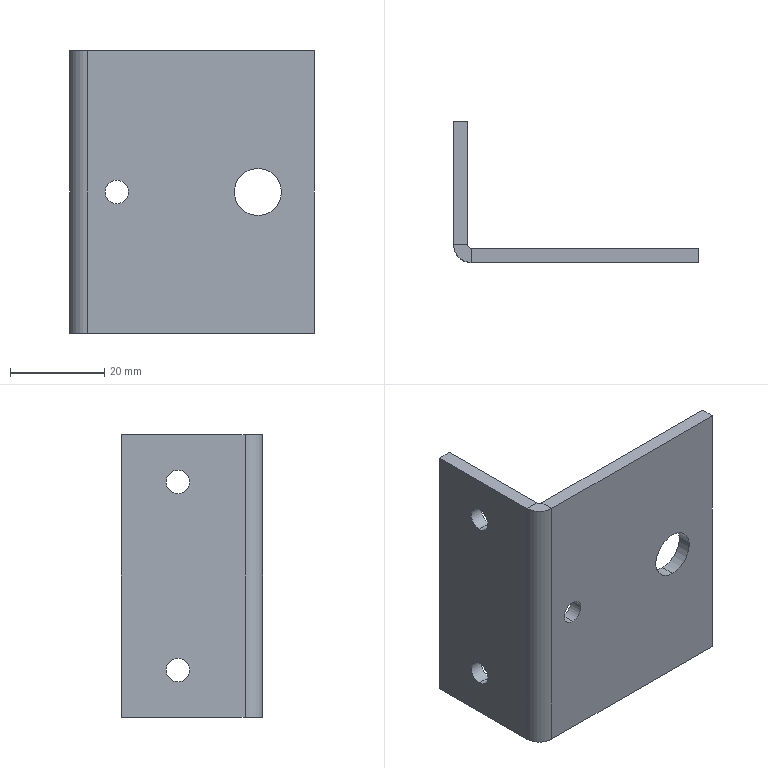Part | NX | features BREP 1 | 1 solid | 22 faces | box 52 x 30 x 60 mm | volume 13635 mm3 | plane 12 | cylinder 10 | commonest cylinder face diameters 5 x6 10 x2 1.473 x1 7.473 x1
STEP:
#1=CARTESIAN_POINT('',(-52.,18.,-22.5));
#2=VERTEX_POINT('',#1);
#3=CARTESIAN_POINT('',(-49.,18.,-22.5));
#4=VERTEX_POINT('',#3);
#5=CARTESIAN_POINT('',(-52.,18.,-22.5));
#6=DIRECTION('',(-1.,0.,0.));
#7=VECTOR('',#6,1000.);
#8=LINE('',#5,#7);
#9=EDGE_CURVE('',#2,#4,#8,.F.);
#10=ORIENTED_EDGE('',*,*,#9,.T.);
#11=CARTESIAN_POINT('',(-49.,18.,-17.5));
#12=VERTEX_POINT('',#11);
#13=CARTESIAN_POINT('',(-49.,18.,-20.));
#14=DIRECTION('',(-1.,0.,0.));
#15=DIRECTION('',(0.,-1.,0.));
#16=AXIS2_PLACEMENT_3D('',#13,#14,#15);
#17=CIRCLE('',#16,2.5);
#18=EDGE_CURVE('',#12,#4,#17,.T.);
#19=ORIENTED_EDGE('',*,*,#18,.F.);
#20=CARTESIAN_POINT('',(-52.,18.,-17.5));
#21=VERTEX_POINT('',#20);
#22=CARTESIAN_POINT('',(-52.,18.,-17.5));
#23=DIRECTION('',(-1.,0.,0.));
#24=VECTOR('',#23,1000.);
#25=LINE('',#22,#24);
#26=EDGE_CURVE('',#21,#12,#25,.F.);
#27=ORIENTED_EDGE('',*,*,#26,.F.);
#28=CARTESIAN_POINT('',(-52.,18.,-20.));
#29=DIRECTION('',(-1.,0.,0.));
#30=DIRECTION('',(0.,0.,1.));
#31=AXIS2_PLACEMENT_3D('',#28,#29,#30);
#32=CIRCLE('',#31,2.5);
#33=EDGE_CURVE('',#21,#2,#32,.T.);
#34=ORIENTED_EDGE('',*,*,#33,.T.);
#35=EDGE_LOOP('',(#10,#19,#27,#34));
#36=FACE_BOUND('',#35,.T.);
#37=CARTESIAN_POINT('',(-52.,18.,-20.));
#38=DIRECTION('',(-1.,0.,0.));
#39=DIRECTION('',(0.,0.,1.));
#40=AXIS2_PLACEMENT_3D('',#37,#38,#39);
#41=CYLINDRICAL_SURFACE('',#40,2.5);
#42=ADVANCED_FACE('',(#36),#41,.F.);
#43=CARTESIAN_POINT('',(-52.,18.,17.5));
#44=VERTEX_POINT('',#43);
#45=CARTESIAN_POINT('',(-49.,18.,17.5));
#46=VERTEX_POINT('',#45);
#47=CARTESIAN_POINT('',(-52.,18.,17.5));
#48=DIRECTION('',(-1.,0.,0.));
#49=VECTOR('',#48,1000.);
#50=LINE('',#47,#49);
#51=EDGE_CURVE('',#44,#46,#50,.F.);
#52=ORIENTED_EDGE('',*,*,#51,.T.);
#53=CARTESIAN_POINT('',(-49.,18.,22.5));
#54=VERTEX_POINT('',#53);
#55=CARTESIAN_POINT('',(-49.,18.,20.));
#56=DIRECTION('',(-1.,0.,0.));
#57=DIRECTION('',(0.,-1.,0.));
#58=AXIS2_PLACEMENT_3D('',#55,#56,#57);
#59=CIRCLE('',#58,2.5);
#60=EDGE_CURVE('',#54,#46,#59,.T.);
#61=ORIENTED_EDGE('',*,*,#60,.F.);
#62=CARTESIAN_POINT('',(-52.,18.,22.5));
#63=VERTEX_POINT('',#62);
#64=CARTESIAN_POINT('',(-52.,18.,22.5));
#65=DIRECTION('',(-1.,0.,0.));
#66=VECTOR('',#65,1000.);
#67=LINE('',#64,#66);
#68=EDGE_CURVE('',#63,#54,#67,.F.);
#69=ORIENTED_EDGE('',*,*,#68,.F.);
#70=CARTESIAN_POINT('',(-52.,18.,20.));
#71=DIRECTION('',(-1.,0.,0.));
#72=DIRECTION('',(0.,0.,1.));
#73=AXIS2_PLACEMENT_3D('',#70,#71,#72);
#74=CIRCLE('',#73,2.5);
#75=EDGE_CURVE('',#63,#44,#74,.T.);
#76=ORIENTED_EDGE('',*,*,#75,.T.);
#77=EDGE_LOOP('',(#52,#61,#69,#76));
#78=FACE_BOUND('',#77,.T.);
#79=CARTESIAN_POINT('',(-52.,18.,20.));
#80=DIRECTION('',(-1.,0.,0.));
#81=DIRECTION('',(0.,0.,1.));
#82=AXIS2_PLACEMENT_3D('',#79,#80,#81);
#83=CYLINDRICAL_SURFACE('',#82,2.5);
#84=ADVANCED_FACE('',(#78),#83,.F.);
#85=CARTESIAN_POINT('',(-42.,3.,2.5));
#86=VERTEX_POINT('',#85);
#87=CARTESIAN_POINT('',(-42.,0.,2.5));
#88=VERTEX_POINT('',#87);
#89=CARTESIAN_POINT('',(-42.,0.,2.5));
#90=DIRECTION('',(0.,-1.,0.));
#91=VECTOR('',#90,1000.);
#92=LINE('',#89,#91);
#93=EDGE_CURVE('',#86,#88,#92,.T.);
#94=ORIENTED_EDGE('',*,*,#93,.F.);
#95=CARTESIAN_POINT('',(-42.,3.,-2.5));
#96=VERTEX_POINT('',#95);
#97=CARTESIAN_POINT('',(-42.,3.,0.));
#98=DIRECTION('',(0.,-1.,0.));
#99=DIRECTION('',(1.,0.,0.));
#100=AXIS2_PLACEMENT_3D('',#97,#98,#99);
#101=CIRCLE('',#100,2.5);
#102=EDGE_CURVE('',#96,#86,#101,.T.);
#103=ORIENTED_EDGE('',*,*,#102,.F.);
#104=CARTESIAN_POINT('',(-42.,0.,-2.5));
#105=VERTEX_POINT('',#104);
#106=CARTESIAN_POINT('',(-42.,0.,-2.5));
#107=DIRECTION('',(0.,-1.,0.));
#108=VECTOR('',#107,1000.);
#109=LINE('',#106,#108);
#110=EDGE_CURVE('',#96,#105,#109,.T.);
#111=ORIENTED_EDGE('',*,*,#110,.T.);
#112=CARTESIAN_POINT('',(-42.,0.,0.));
#113=DIRECTION('',(0.,-1.,0.));
#114=DIRECTION('',(0.,0.,-1.));
#115=AXIS2_PLACEMENT_3D('',#112,#113,#114);
#116=CIRCLE('',#115,2.5);
#117=EDGE_CURVE('',#105,#88,#116,.T.);
#118=ORIENTED_EDGE('',*,*,#117,.T.);
#119=EDGE_LOOP('',(#94,#103,#111,#118));
#120=FACE_BOUND('',#119,.T.);
#121=CARTESIAN_POINT('',(-42.,0.,0.));
#122=DIRECTION('',(0.,-1.,0.));
#123=DIRECTION('',(0.,0.,-1.));
#124=AXIS2_PLACEMENT_3D('',#121,#122,#123);
#125=CYLINDRICAL_SURFACE('',#124,2.5);
#126=ADVANCED_FACE('',(#120),#125,.F.);
#127=CARTESIAN_POINT('',(-12.,3.,-5.));
#128=VERTEX_POINT('',#127);
#129=CARTESIAN_POINT('',(-12.,0.,-5.));
#130=VERTEX_POINT('',#129);
#131=CARTESIAN_POINT('',(-12.,3.,-5.));
#132=DIRECTION('',(0.,1.,0.));
#133=VECTOR('',#132,1000.);
#134=LINE('',#131,#133);
#135=EDGE_CURVE('',#128,#130,#134,.F.);
#136=ORIENTED_EDGE('',*,*,#135,.T.);
#137=CARTESIAN_POINT('',(-12.,0.,5.));
#138=VERTEX_POINT('',#137);
#139=CARTESIAN_POINT('',(-12.,0.,0.));
#140=DIRECTION('',(0.,1.,0.));
#141=DIRECTION('',(0.,0.,1.));
#142=AXIS2_PLACEMENT_3D('',#139,#140,#141);
#143=CIRCLE('',#142,5.);
#144=EDGE_CURVE('',#138,#130,#143,.T.);
#145=ORIENTED_EDGE('',*,*,#144,.F.);
#146=CARTESIAN_POINT('',(-12.,3.,5.));
#147=VERTEX_POINT('',#146);
#148=CARTESIAN_POINT('',(-12.,3.,5.));
#149=DIRECTION('',(0.,1.,0.));
#150=VECTOR('',#149,1000.);
#151=LINE('',#148,#150);
#152=EDGE_CURVE('',#147,#138,#151,.F.);
#153=ORIENTED_EDGE('',*,*,#152,.F.);
#154=CARTESIAN_POINT('',(-12.,3.,0.));
#155=DIRECTION('',(0.,1.,0.));
#156=DIRECTION('',(0.,0.,1.));
#157=AXIS2_PLACEMENT_3D('',#154,#155,#156);
#158=CIRCLE('',#157,5.);
#159=EDGE_CURVE('',#147,#128,#158,.T.);
#160=ORIENTED_EDGE('',*,*,#159,.T.);
#161=EDGE_LOOP('',(#136,#145,#153,#160));
#162=FACE_BOUND('',#161,.T.);
#163=CARTESIAN_POINT('',(-12.,3.,0.));
#164=DIRECTION('',(0.,1.,0.));
#165=DIRECTION('',(0.,0.,1.));
#166=AXIS2_PLACEMENT_3D('',#163,#164,#165);
#167=CYLINDRICAL_SURFACE('',#166,5.);
#168=ADVANCED_FACE('',(#162),#167,.F.);
#169=CARTESIAN_POINT('',(-49.,3.737,-30.));
#170=VERTEX_POINT('',#169);
#171=CARTESIAN_POINT('',(-49.,30.,-30.));
#172=VERTEX_POINT('',#171);
#173=CARTESIAN_POINT('',(-49.,0.,-30.));
#174=DIRECTION('',(0.,1.,0.));
#175=VECTOR('',#174,1000.);
#176=LINE('',#173,#175);
#177=EDGE_CURVE('',#170,#172,#176,.T.);
#178=ORIENTED_EDGE('',*,*,#177,.F.);
#179=CARTESIAN_POINT('',(-52.,3.737,-30.));
#180=VERTEX_POINT('',#179);
#181=CARTESIAN_POINT('',(-49.,3.737,-30.));
#182=DIRECTION('',(-1.,0.,0.));
#183=VECTOR('',#182,1000.);
#184=LINE('',#181,#183);
#185=EDGE_CURVE('',#170,#180,#184,.T.);
#186=ORIENTED_EDGE('',*,*,#185,.T.);
#187=CARTESIAN_POINT('',(-52.,30.,-30.));
#188=VERTEX_POINT('',#187);
#189=CARTESIAN_POINT('',(-52.,0.,-30.));
#190=DIRECTION('',(0.,1.,0.));
#191=VECTOR('',#190,1000.);
#192=LINE('',#189,#191);
#193=EDGE_CURVE('',#180,#188,#192,.T.);
#194=ORIENTED_EDGE('',*,*,#193,.T.);
#195=CARTESIAN_POINT('',(-52.,30.,-30.));
#196=DIRECTION('',(1.,0.,0.));
#197=VECTOR('',#196,1000.);
#198=LINE('',#195,#197);
#199=EDGE_CURVE('',#188,#172,#198,.T.);
#200=ORIENTED_EDGE('',*,*,#199,.T.);
#201=EDGE_LOOP('',(#178,#186,#194,#200));
#202=FACE_BOUND('',#201,.T.);
#203=CARTESIAN_POINT('',(-48.263,3.737,-30.));
#204=DIRECTION('',(0.,0.,1.));
#205=DIRECTION('',(1.,0.,0.));
#206=AXIS2_PLACEMENT_3D('',#203,#204,#205);
#207=PLANE('',#206);
#208=ADVANCED_FACE('',(#202),#207,.F.);
#209=CARTESIAN_POINT('',(0.,3.,30.));
#210=VERTEX_POINT('',#209);
#211=CARTESIAN_POINT('',(-48.263,3.,30.));
#212=VERTEX_POINT('',#211);
#213=CARTESIAN_POINT('',(0.,3.,30.));
#214=DIRECTION('',(-1.,0.,0.));
#215=VECTOR('',#214,1000.);
#216=LINE('',#213,#215);
#217=EDGE_CURVE('',#210,#212,#216,.T.);
#218=ORIENTED_EDGE('',*,*,#217,.T.);
#219=CARTESIAN_POINT('',(-48.263,0.,30.));
#220=VERTEX_POINT('',#219);
#221=CARTESIAN_POINT('',(-48.263,3.,30.));
#222=DIRECTION('',(0.,-1.,0.));
#223=VECTOR('',#222,1000.);
#224=LINE('',#221,#223);
#225=EDGE_CURVE('',#212,#220,#224,.T.);
#226=ORIENTED_EDGE('',*,*,#225,.T.);
#227=CARTESIAN_POINT('',(0.,0.,30.));
#228=VERTEX_POINT('',#227);
#229=CARTESIAN_POINT('',(0.,0.,30.));
#230=DIRECTION('',(-1.,0.,0.));
#231=VECTOR('',#230,1000.);
#232=LINE('',#229,#231);
#233=EDGE_CURVE('',#228,#220,#232,.T.);
#234=ORIENTED_EDGE('',*,*,#233,.F.);
#235=CARTESIAN_POINT('',(0.,3.,30.));
#236=DIRECTION('',(0.,-1.,0.));
#237=VECTOR('',#236,1000.);
#238=LINE('',#235,#237);
#239=EDGE_CURVE('',#210,#228,#238,.T.);
#240=ORIENTED_EDGE('',*,*,#239,.F.);
#241=EDGE_LOOP('',(#218,#226,#234,#240));
#242=FACE_BOUND('',#241,.T.);
#243=CARTESIAN_POINT('',(-48.263,3.737,30.));
#244=DIRECTION('',(0.,0.,1.));
#245=DIRECTION('',(1.,0.,0.));
#246=AXIS2_PLACEMENT_3D('',#243,#244,#245);
#247=PLANE('',#246);
#248=ADVANCED_FACE('',(#242),#247,.T.);
#249=CARTESIAN_POINT('',(-48.263,3.,-30.));
#250=VERTEX_POINT('',#249);
#251=CARTESIAN_POINT('',(-48.263,3.737,-30.));
#252=DIRECTION('',(0.,0.,-1.));
#253=DIRECTION('',(1.,0.,0.));
#254=AXIS2_PLACEMENT_3D('',#251,#252,#253);
#255=CIRCLE('',#254,0.7366);
#256=EDGE_CURVE('',#250,#170,#255,.T.);
#257=ORIENTED_EDGE('',*,*,#256,.T.);
#258=CARTESIAN_POINT('',(-49.,3.737,30.));
#259=VERTEX_POINT('',#258);
#260=CARTESIAN_POINT('',(-49.,3.737,30.));
#261=DIRECTION('',(0.,0.,-1.));
#262=VECTOR('',#261,1000.);
#263=LINE('',#260,#262);
#264=EDGE_CURVE('',#259,#170,#263,.T.);
#265=ORIENTED_EDGE('',*,*,#264,.F.);
#266=CARTESIAN_POINT('',(-48.263,3.737,30.));
#267=DIRECTION('',(0.,0.,-1.));
#268=DIRECTION('',(1.,0.,0.));
#269=AXIS2_PLACEMENT_3D('',#266,#267,#268);
#270=CIRCLE('',#269,0.7366);
#271=EDGE_CURVE('',#212,#259,#270,.T.);
#272=ORIENTED_EDGE('',*,*,#271,.F.);
#273=CARTESIAN_POINT('',(-48.263,3.,30.));
#274=DIRECTION('',(0.,0.,-1.));
#275=VECTOR('',#274,1000.);
#276=LINE('',#273,#275);
#277=EDGE_CURVE('',#212,#250,#276,.T.);
#278=ORIENTED_EDGE('',*,*,#277,.T.);
#279=EDGE_LOOP('',(#257,#265,#272,#278));
#280=FACE_BOUND('',#279,.T.);
#281=CARTESIAN_POINT('',(-48.263,3.737,30.));
#282=DIRECTION('',(0.,0.,-1.));
#283=DIRECTION('',(-1.,0.,0.));
#284=AXIS2_PLACEMENT_3D('',#281,#282,#283);
#285=CYLINDRICAL_SURFACE('',#284,0.7366);
#286=ADVANCED_FACE('',(#280),#285,.F.);
#287=CARTESIAN_POINT('',(0.,3.,-30.));
#288=VERTEX_POINT('',#287);
#289=CARTESIAN_POINT('',(0.,3.,-30.));
#290=DIRECTION('',(-1.,0.,0.));
#291=VECTOR('',#290,1000.);
#292=LINE('',#289,#291);
#293=EDGE_CURVE('',#288,#250,#292,.T.);
#294=ORIENTED_EDGE('',*,*,#293,.T.);
#295=ORIENTED_EDGE('',*,*,#277,.F.);
#296=ORIENTED_EDGE('',*,*,#217,.F.);
#297=CARTESIAN_POINT('',(0.,3.,30.));
#298=DIRECTION('',(0.,0.,-1.));
#299=VECTOR('',#298,1000.);
#300=LINE('',#297,#299);
#301=EDGE_CURVE('',#210,#288,#300,.T.);
#302=ORIENTED_EDGE('',*,*,#301,.T.);
#303=EDGE_LOOP('',(#294,#295,#296,#302));
#304=FACE_BOUND('',#303,.T.);
#305=ORIENTED_EDGE('',*,*,#159,.F.);
#306=CARTESIAN_POINT('',(-12.,3.,0.));
#307=DIRECTION('',(0.,1.,0.));
#308=DIRECTION('',(0.,0.,1.));
#309=AXIS2_PLACEMENT_3D('',#306,#307,#308);
#310=CIRCLE('',#309,5.);
#311=EDGE_CURVE('',#128,#147,#310,.T.);
#312=ORIENTED_EDGE('',*,*,#311,.F.);
#313=EDGE_LOOP('',(#305,#312));
#314=FACE_BOUND('',#313,.T.);
#315=ORIENTED_EDGE('',*,*,#102,.T.);
#316=CARTESIAN_POINT('',(-42.,3.,0.));
#317=DIRECTION('',(0.,-1.,0.));
#318=DIRECTION('',(1.,0.,0.));
#319=AXIS2_PLACEMENT_3D('',#316,#317,#318);
#320=CIRCLE('',#319,2.5);
#321=EDGE_CURVE('',#86,#96,#320,.T.);
#322=ORIENTED_EDGE('',*,*,#321,.T.);
#323=EDGE_LOOP('',(#315,#322));
#324=FACE_BOUND('',#323,.T.);
#325=CARTESIAN_POINT('',(0.,3.,30.));
#326=DIRECTION('',(0.,-1.,0.));
#327=DIRECTION('',(1.,0.,0.));
#328=AXIS2_PLACEMENT_3D('',#325,#326,#327);
#329=PLANE('',#328);
#330=ADVANCED_FACE('',(#304,#314,#324),#329,.F.);
#331=CARTESIAN_POINT('',(0.,0.,-30.));
#332=VERTEX_POINT('',#331);
#333=CARTESIAN_POINT('',(0.,3.,-30.));
#334=DIRECTION('',(0.,-1.,0.));
#335=VECTOR('',#334,1000.);
#336=LINE('',#333,#335);
#337=EDGE_CURVE('',#288,#332,#336,.T.);
#338=ORIENTED_EDGE('',*,*,#337,.F.);
#339=ORIENTED_EDGE('',*,*,#301,.F.);
#340=ORIENTED_EDGE('',*,*,#239,.T.);
#341=CARTESIAN_POINT('',(0.,0.,30.));
#342=DIRECTION('',(0.,0.,-1.));
#343=VECTOR('',#342,1000.);
#344=LINE('',#341,#343);
#345=EDGE_CURVE('',#228,#332,#344,.T.);
#346=ORIENTED_EDGE('',*,*,#345,.T.);
#347=EDGE_LOOP('',(#338,#339,#340,#346));
#348=FACE_BOUND('',#347,.T.);
#349=CARTESIAN_POINT('',(0.,3.,30.));
#350=DIRECTION('',(1.,0.,0.));
#351=DIRECTION('',(0.,1.,0.));
#352=AXIS2_PLACEMENT_3D('',#349,#350,#351);
#353=PLANE('',#352);
#354=ADVANCED_FACE('',(#348),#353,.T.);
#355=CARTESIAN_POINT('',(-48.263,0.,-30.));
#356=VERTEX_POINT('',#355);
#357=CARTESIAN_POINT('',(0.,0.,-30.));
#358=DIRECTION('',(-1.,0.,0.));
#359=VECTOR('',#358,1000.);
#360=LINE('',#357,#359);
#361=EDGE_CURVE('',#332,#356,#360,.T.);
#362=ORIENTED_EDGE('',*,*,#361,.F.);
#363=ORIENTED_EDGE('',*,*,#345,.F.);
#364=ORIENTED_EDGE('',*,*,#233,.T.);
#365=CARTESIAN_POINT('',(-48.263,0.,30.));
#366=DIRECTION('',(0.,0.,-1.));
#367=VECTOR('',#366,1000.);
#368=LINE('',#365,#367);
#369=EDGE_CURVE('',#220,#356,#368,.T.);
#370=ORIENTED_EDGE('',*,*,#369,.T.);
#371=EDGE_LOOP('',(#362,#363,#364,#370));
#372=FACE_BOUND('',#371,.T.);
#373=ORIENTED_EDGE('',*,*,#144,.T.);
#374=CARTESIAN_POINT('',(-12.,0.,0.));
#375=DIRECTION('',(0.,1.,0.));
#376=DIRECTION('',(0.,0.,1.));
#377=AXIS2_PLACEMENT_3D('',#374,#375,#376);
#378=CIRCLE('',#377,5.);
#379=EDGE_CURVE('',#130,#138,#378,.T.);
#380=ORIENTED_EDGE('',*,*,#379,.T.);
#381=EDGE_LOOP('',(#373,#380));
#382=FACE_BOUND('',#381,.T.);
#383=ORIENTED_EDGE('',*,*,#117,.F.);
#384=CARTESIAN_POINT('',(-42.,0.,0.));
#385=DIRECTION('',(0.,-1.,0.));
#386=DIRECTION('',(0.,0.,-1.));
#387=AXIS2_PLACEMENT_3D('',#384,#385,#386);
#388=CIRCLE('',#387,2.5);
#389=EDGE_CURVE('',#88,#105,#388,.T.);
#390=ORIENTED_EDGE('',*,*,#389,.F.);
#391=EDGE_LOOP('',(#383,#390));
#392=FACE_BOUND('',#391,.T.);
#393=CARTESIAN_POINT('',(0.,0.,30.));
#394=DIRECTION('',(0.,-1.,0.));
#395=DIRECTION('',(1.,0.,0.));
#396=AXIS2_PLACEMENT_3D('',#393,#394,#395);
#397=PLANE('',#396);
#398=ADVANCED_FACE('',(#372,#382,#392),#397,.T.);
#399=CARTESIAN_POINT('',(-48.263,3.737,-30.));
#400=DIRECTION('',(0.,0.,-1.));
#401=DIRECTION('',(1.,0.,0.));
#402=AXIS2_PLACEMENT_3D('',#399,#400,#401);
#403=CIRCLE('',#402,3.737);
#404=EDGE_CURVE('',#356,#180,#403,.T.);
#405=ORIENTED_EDGE('',*,*,#404,.F.);
#406=ORIENTED_EDGE('',*,*,#369,.F.);
#407=CARTESIAN_POINT('',(-52.,3.737,30.));
#408=VERTEX_POINT('',#407);
#409=CARTESIAN_POINT('',(-48.263,3.737,30.));
#410=DIRECTION('',(0.,0.,-1.));
#411=DIRECTION('',(1.,0.,0.));
#412=AXIS2_PLACEMENT_3D('',#409,#410,#411);
#413=CIRCLE('',#412,3.737);
#414=EDGE_CURVE('',#220,#408,#413,.T.);
#415=ORIENTED_EDGE('',*,*,#414,.T.);
#416=CARTESIAN_POINT('',(-52.,3.737,30.));
#417=DIRECTION('',(0.,0.,-1.));
#418=VECTOR('',#417,1000.);
#419=LINE('',#416,#418);
#420=EDGE_CURVE('',#408,#180,#419,.T.);
#421=ORIENTED_EDGE('',*,*,#420,.T.);
#422=EDGE_LOOP('',(#405,#406,#415,#421));
#423=FACE_BOUND('',#422,.T.);
#424=CARTESIAN_POINT('',(-48.263,3.737,30.));
#425=DIRECTION('',(0.,0.,-1.));
#426=DIRECTION('',(-1.,0.,0.));
#427=AXIS2_PLACEMENT_3D('',#424,#425,#426);
#428=CYLINDRICAL_SURFACE('',#427,3.737);
#429=ADVANCED_FACE('',(#423),#428,.T.);
#430=ORIENTED_EDGE('',*,*,#193,.F.);
#431=ORIENTED_EDGE('',*,*,#420,.F.);
#432=CARTESIAN_POINT('',(-52.,30.,30.));
#433=VERTEX_POINT('',#432);
#434=CARTESIAN_POINT('',(-52.,0.,30.));
#435=DIRECTION('',(0.,1.,0.));
#436=VECTOR('',#435,1000.);
#437=LINE('',#434,#436);
#438=EDGE_CURVE('',#408,#433,#437,.T.);
#439=ORIENTED_EDGE('',*,*,#438,.T.);
#440=CARTESIAN_POINT('',(-52.,30.,30.));
#441=DIRECTION('',(0.,0.,-1.));
#442=VECTOR('',#441,1000.);
#443=LINE('',#440,#442);
#444=EDGE_CURVE('',#433,#188,#443,.T.);
#445=ORIENTED_EDGE('',*,*,#444,.T.);
#446=EDGE_LOOP('',(#430,#431,#439,#445));
#447=FACE_BOUND('',#446,.T.);
#448=ORIENTED_EDGE('',*,*,#75,.F.);
#449=CARTESIAN_POINT('',(-52.,18.,20.));
#450=DIRECTION('',(-1.,0.,0.));
#451=DIRECTION('',(0.,0.,1.));
#452=AXIS2_PLACEMENT_3D('',#449,#450,#451);
#453=CIRCLE('',#452,2.5);
#454=EDGE_CURVE('',#44,#63,#453,.T.);
#455=ORIENTED_EDGE('',*,*,#454,.F.);
#456=EDGE_LOOP('',(#448,#455));
#457=FACE_BOUND('',#456,.T.);
#458=ORIENTED_EDGE('',*,*,#33,.F.);
#459=CARTESIAN_POINT('',(-52.,18.,-20.));
#460=DIRECTION('',(-1.,0.,0.));
#461=DIRECTION('',(0.,0.,1.));
#462=AXIS2_PLACEMENT_3D('',#459,#460,#461);
#463=CIRCLE('',#462,2.5);
#464=EDGE_CURVE('',#2,#21,#463,.T.);
#465=ORIENTED_EDGE('',*,*,#464,.F.);
#466=EDGE_LOOP('',(#458,#465));
#467=FACE_BOUND('',#466,.T.);
#468=CARTESIAN_POINT('',(-52.,0.,30.));
#469=DIRECTION('',(-1.,0.,0.));
#470=DIRECTION('',(0.,-1.,0.));
#471=AXIS2_PLACEMENT_3D('',#468,#469,#470);
#472=PLANE('',#471);
#473=ADVANCED_FACE('',(#447,#457,#467),#472,.T.);
#474=ORIENTED_EDGE('',*,*,#199,.F.);
#475=ORIENTED_EDGE('',*,*,#444,.F.);
#476=CARTESIAN_POINT('',(-49.,30.,30.));
#477=VERTEX_POINT('',#476);
#478=CARTESIAN_POINT('',(-52.,30.,30.));
#479=DIRECTION('',(1.,0.,0.));
#480=VECTOR('',#479,1000.);
#481=LINE('',#478,#480);
#482=EDGE_CURVE('',#433,#477,#481,.T.);
#483=ORIENTED_EDGE('',*,*,#482,.T.);
#484=CARTESIAN_POINT('',(-49.,30.,30.));
#485=DIRECTION('',(0.,0.,-1.));
#486=VECTOR('',#485,1000.);
#487=LINE('',#484,#486);
#488=EDGE_CURVE('',#477,#172,#487,.T.);
#489=ORIENTED_EDGE('',*,*,#488,.T.);
#490=EDGE_LOOP('',(#474,#475,#483,#489));
#491=FACE_BOUND('',#490,.T.);
#492=CARTESIAN_POINT('',(-52.,30.,30.));
#493=DIRECTION('',(0.,1.,0.));
#494=DIRECTION('',(0.,0.,1.));
#495=AXIS2_PLACEMENT_3D('',#492,#493,#494);
#496=PLANE('',#495);
#497=ADVANCED_FACE('',(#491),#496,.T.);
#498=ORIENTED_EDGE('',*,*,#177,.T.);
#499=ORIENTED_EDGE('',*,*,#488,.F.);
#500=CARTESIAN_POINT('',(-49.,0.,30.));
#501=DIRECTION('',(0.,1.,0.));
#502=VECTOR('',#501,1000.);
#503=LINE('',#500,#502);
#504=EDGE_CURVE('',#259,#477,#503,.T.);
#505=ORIENTED_EDGE('',*,*,#504,.F.);
#506=ORIENTED_EDGE('',*,*,#264,.T.);
#507=EDGE_LOOP('',(#498,#499,#505,#506));
#508=FACE_BOUND('',#507,.T.);
#509=ORIENTED_EDGE('',*,*,#60,.T.);
#510=CARTESIAN_POINT('',(-49.,18.,20.));
#511=DIRECTION('',(-1.,0.,0.));
#512=DIRECTION('',(0.,-1.,0.));
#513=AXIS2_PLACEMENT_3D('',#510,#511,#512);
#514=CIRCLE('',#513,2.5);
#515=EDGE_CURVE('',#46,#54,#514,.T.);
#516=ORIENTED_EDGE('',*,*,#515,.T.);
#517=EDGE_LOOP('',(#509,#516));
#518=FACE_BOUND('',#517,.T.);
#519=ORIENTED_EDGE('',*,*,#18,.T.);
#520=CARTESIAN_POINT('',(-49.,18.,-20.));
#521=DIRECTION('',(-1.,0.,0.));
#522=DIRECTION('',(0.,-1.,0.));
#523=AXIS2_PLACEMENT_3D('',#520,#521,#522);
#524=CIRCLE('',#523,2.5);
#525=EDGE_CURVE('',#4,#12,#524,.T.);
#526=ORIENTED_EDGE('',*,*,#525,.T.);
#527=EDGE_LOOP('',(#519,#526));
#528=FACE_BOUND('',#527,.T.);
#529=CARTESIAN_POINT('',(-49.,0.,30.));
#530=DIRECTION('',(-1.,0.,0.));
#531=DIRECTION('',(0.,-1.,0.));
#532=AXIS2_PLACEMENT_3D('',#529,#530,#531);
#533=PLANE('',#532);
#534=ADVANCED_FACE('',(#508,#518,#528),#533,.F.);
#535=ORIENTED_EDGE('',*,*,#361,.T.);
#536=CARTESIAN_POINT('',(-48.263,0.,-30.));
#537=DIRECTION('',(0.,1.,0.));
#538=VECTOR('',#537,1000.);
#539=LINE('',#536,#538);
#540=EDGE_CURVE('',#356,#250,#539,.T.);
#541=ORIENTED_EDGE('',*,*,#540,.T.);
#542=ORIENTED_EDGE('',*,*,#293,.F.);
#543=ORIENTED_EDGE('',*,*,#337,.T.);
#544=EDGE_LOOP('',(#535,#541,#542,#543));
#545=FACE_BOUND('',#544,.T.);
#546=CARTESIAN_POINT('',(-49.,3.737,-30.));
#547=DIRECTION('',(0.,0.,-1.));
#548=DIRECTION('',(-1.,0.,0.));
#549=AXIS2_PLACEMENT_3D('',#546,#547,#548);
#550=PLANE('',#549);
#551=ADVANCED_FACE('',(#545),#550,.T.);
#552=ORIENTED_EDGE('',*,*,#540,.F.);
#553=ORIENTED_EDGE('',*,*,#404,.T.);
#554=ORIENTED_EDGE('',*,*,#185,.F.);
#555=ORIENTED_EDGE('',*,*,#256,.F.);
#556=EDGE_LOOP('',(#552,#553,#554,#555));
#557=FACE_BOUND('',#556,.T.);
#558=CARTESIAN_POINT('',(-48.263,0.,-30.));
#559=DIRECTION('',(0.,0.,-1.));
#560=DIRECTION('',(-1.,0.,0.));
#561=AXIS2_PLACEMENT_3D('',#558,#559,#560);
#562=PLANE('',#561);
#563=ADVANCED_FACE('',(#557),#562,.T.);
#564=ORIENTED_EDGE('',*,*,#438,.F.);
#565=CARTESIAN_POINT('',(-52.,3.737,30.));
#566=DIRECTION('',(1.,0.,0.));
#567=VECTOR('',#566,1000.);
#568=LINE('',#565,#567);
#569=EDGE_CURVE('',#408,#259,#568,.T.);
#570=ORIENTED_EDGE('',*,*,#569,.T.);
#571=ORIENTED_EDGE('',*,*,#504,.T.);
#572=ORIENTED_EDGE('',*,*,#482,.F.);
#573=EDGE_LOOP('',(#564,#570,#571,#572));
#574=FACE_BOUND('',#573,.T.);
#575=CARTESIAN_POINT('',(-48.263,3.,30.));
#576=DIRECTION('',(0.,0.,1.));
#577=DIRECTION('',(1.,0.,0.));
#578=AXIS2_PLACEMENT_3D('',#575,#576,#577);
#579=PLANE('',#578);
#580=ADVANCED_FACE('',(#574),#579,.T.);
#581=ORIENTED_EDGE('',*,*,#569,.F.);
#582=ORIENTED_EDGE('',*,*,#414,.F.);
#583=ORIENTED_EDGE('',*,*,#225,.F.);
#584=ORIENTED_EDGE('',*,*,#271,.T.);
#585=EDGE_LOOP('',(#581,#582,#583,#584));
#586=FACE_BOUND('',#585,.T.);
#587=CARTESIAN_POINT('',(-52.,3.737,30.));
#588=DIRECTION('',(0.,0.,1.));
#589=DIRECTION('',(1.,0.,0.));
#590=AXIS2_PLACEMENT_3D('',#587,#588,#589);
#591=PLANE('',#590);
#592=ADVANCED_FACE('',(#586),#591,.T.);
#593=ORIENTED_EDGE('',*,*,#379,.F.);
#594=ORIENTED_EDGE('',*,*,#135,.F.);
#595=ORIENTED_EDGE('',*,*,#311,.T.);
#596=ORIENTED_EDGE('',*,*,#152,.T.);
#597=EDGE_LOOP('',(#593,#594,#595,#596));
#598=FACE_BOUND('',#597,.T.);
#599=CARTESIAN_POINT('',(-12.,3.,0.));
#600=DIRECTION('',(0.,1.,0.));
#601=DIRECTION('',(0.,0.,1.));
#602=AXIS2_PLACEMENT_3D('',#599,#600,#601);
#603=CYLINDRICAL_SURFACE('',#602,5.);
#604=ADVANCED_FACE('',(#598),#603,.F.);
#605=ORIENTED_EDGE('',*,*,#321,.F.);
#606=ORIENTED_EDGE('',*,*,#93,.T.);
#607=ORIENTED_EDGE('',*,*,#389,.T.);
#608=ORIENTED_EDGE('',*,*,#110,.F.);
#609=EDGE_LOOP('',(#605,#606,#607,#608));
#610=FACE_BOUND('',#609,.T.);
#611=CARTESIAN_POINT('',(-42.,0.,0.));
#612=DIRECTION('',(0.,-1.,0.));
#613=DIRECTION('',(0.,0.,-1.));
#614=AXIS2_PLACEMENT_3D('',#611,#612,#613);
#615=CYLINDRICAL_SURFACE('',#614,2.5);
#616=ADVANCED_FACE('',(#610),#615,.F.);
#617=ORIENTED_EDGE('',*,*,#515,.F.);
#618=ORIENTED_EDGE('',*,*,#51,.F.);
#619=ORIENTED_EDGE('',*,*,#454,.T.);
#620=ORIENTED_EDGE('',*,*,#68,.T.);
#621=EDGE_LOOP('',(#617,#618,#619,#620));
#622=FACE_BOUND('',#621,.T.);
#623=CARTESIAN_POINT('',(-52.,18.,20.));
#624=DIRECTION('',(-1.,0.,0.));
#625=DIRECTION('',(0.,0.,1.));
#626=AXIS2_PLACEMENT_3D('',#623,#624,#625);
#627=CYLINDRICAL_SURFACE('',#626,2.5);
#628=ADVANCED_FACE('',(#622),#627,.F.);
#629=ORIENTED_EDGE('',*,*,#525,.F.);
#630=ORIENTED_EDGE('',*,*,#9,.F.);
#631=ORIENTED_EDGE('',*,*,#464,.T.);
#632=ORIENTED_EDGE('',*,*,#26,.T.);
#633=EDGE_LOOP('',(#629,#630,#631,#632));
#634=FACE_BOUND('',#633,.T.);
#635=CARTESIAN_POINT('',(-52.,18.,-20.));
#636=DIRECTION('',(-1.,0.,0.));
#637=DIRECTION('',(0.,0.,1.));
#638=AXIS2_PLACEMENT_3D('',#635,#636,#637);
#639=CYLINDRICAL_SURFACE('',#638,2.5);
#640=ADVANCED_FACE('',(#634),#639,.F.);
#641=CLOSED_SHELL('',(#42,#84,#126,#168,#208,#248,#286,#330,#354,#398,#429,#473,#497,#534,#551,#563,#580,#592,#604,#616,#628,#640));
#642=MANIFOLD_SOLID_BREP('',#641);
#643=(LENGTH_UNIT()NAMED_UNIT(*)SI_UNIT(.MILLI.,.METRE.));
#644=UNCERTAINTY_MEASURE_WITH_UNIT(LENGTH_MEASURE(0.00001),#643,'','');
#645=(NAMED_UNIT(*)PLANE_ANGLE_UNIT()SI_UNIT($,.RADIAN.));
#646=(NAMED_UNIT(*)SI_UNIT($,.STERADIAN.)SOLID_ANGLE_UNIT());
#647=(GEOMETRIC_REPRESENTATION_CONTEXT(3)GLOBAL_UNCERTAINTY_ASSIGNED_CONTEXT((#644))GLOBAL_UNIT_ASSIGNED_CONTEXT((#643,#645,#646))REPRESENTATION_CONTEXT('',''));
#648=ADVANCED_BREP_SHAPE_REPRESENTATION('',(#642),#647);